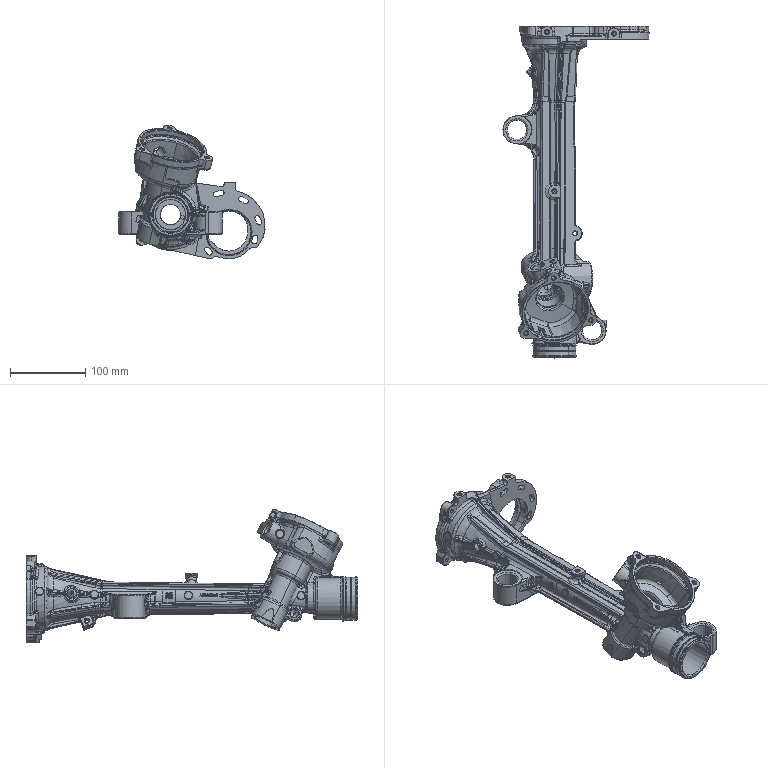Part | SolidWorks | features BaseBody 1 | 1 solid | 3364 faces | volume 689588 mm3 | spline 1513 | plane 603 | cylinder 519 | torus 364 | cone 274 | sphere 91 | commonest cylinder face diameters 2 x78 6 x77 4 x73 4.917 x20 8 x15 10 x15